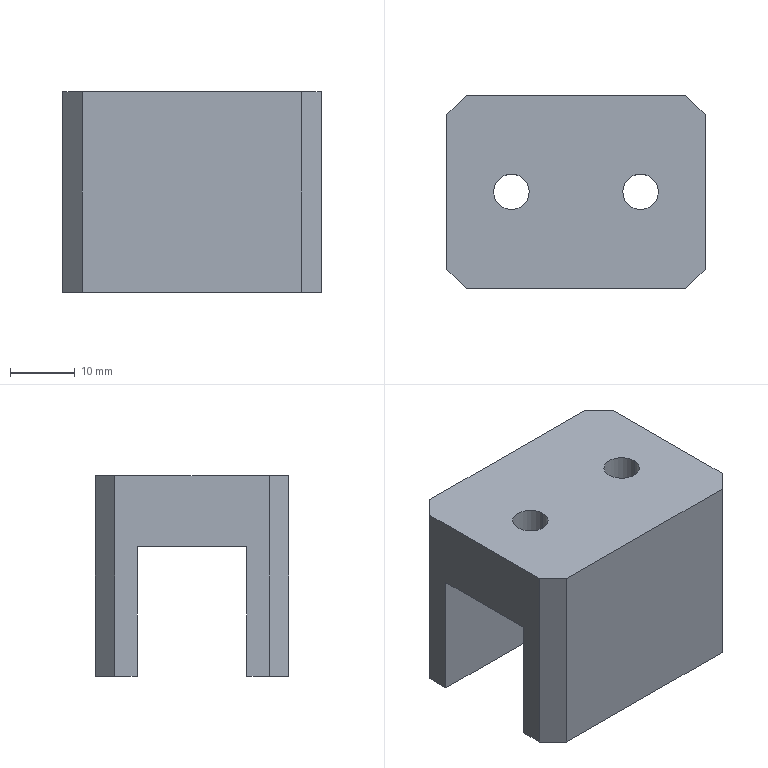Part | Creo | 1 solid | 24 faces | box 40 x 30 x 31 mm | volume 21954 mm3 | plane 16 | cylinder 8 | commonest cylinder face diameters 5.5 x4 9.5 x4
STEP:
#1=CARTESIAN_POINT('',(0.,0.,0.));
#2=DIRECTION('',(0.,0.,1.));
#3=DIRECTION('',(1.,0.,0.));
#4=AXIS2_PLACEMENT_3D('',#1,#2,#3);
#5=CARTESIAN_POINT('',(-118.,-142.,31.5));
#6=VERTEX_POINT('',#5);
#7=CARTESIAN_POINT('',(-152.,-142.,31.5));
#8=VERTEX_POINT('',#7);
#9=CARTESIAN_POINT('',(-118.,-142.,31.5));
#10=DIRECTION('',(-1.,0.,0.));
#11=VECTOR('',#10,34.);
#12=LINE('',#9,#11);
#13=EDGE_CURVE('',#6,#8,#12,.T.);
#14=ORIENTED_EDGE('',*,*,#13,.F.);
#15=CARTESIAN_POINT('',(-115.,-145.,31.5));
#16=VERTEX_POINT('',#15);
#17=CARTESIAN_POINT('',(-115.,-145.,31.5));
#18=DIRECTION('',(-0.7071,0.7071,0.));
#19=VECTOR('',#18,4.243);
#20=LINE('',#17,#19);
#21=EDGE_CURVE('',#16,#6,#20,.T.);
#22=ORIENTED_EDGE('',*,*,#21,.F.);
#23=CARTESIAN_POINT('',(-115.,-169.,31.5));
#24=VERTEX_POINT('',#23);
#25=CARTESIAN_POINT('',(-115.,-169.,31.5));
#26=DIRECTION('',(0.,1.,0.));
#27=VECTOR('',#26,24.);
#28=LINE('',#25,#27);
#29=EDGE_CURVE('',#24,#16,#28,.T.);
#30=ORIENTED_EDGE('',*,*,#29,.F.);
#31=CARTESIAN_POINT('',(-118.,-172.,31.5));
#32=VERTEX_POINT('',#31);
#33=CARTESIAN_POINT('',(-118.,-172.,31.5));
#34=DIRECTION('',(0.7071,0.7071,0.));
#35=VECTOR('',#34,4.243);
#36=LINE('',#33,#35);
#37=EDGE_CURVE('',#32,#24,#36,.T.);
#38=ORIENTED_EDGE('',*,*,#37,.F.);
#39=CARTESIAN_POINT('',(-152.,-172.,31.5));
#40=VERTEX_POINT('',#39);
#41=CARTESIAN_POINT('',(-152.,-172.,31.5));
#42=DIRECTION('',(1.,0.,0.));
#43=VECTOR('',#42,34.);
#44=LINE('',#41,#43);
#45=EDGE_CURVE('',#40,#32,#44,.T.);
#46=ORIENTED_EDGE('',*,*,#45,.F.);
#47=CARTESIAN_POINT('',(-155.,-169.,31.5));
#48=VERTEX_POINT('',#47);
#49=CARTESIAN_POINT('',(-155.,-169.,31.5));
#50=DIRECTION('',(0.7071,-0.7071,0.));
#51=VECTOR('',#50,4.243);
#52=LINE('',#49,#51);
#53=EDGE_CURVE('',#48,#40,#52,.T.);
#54=ORIENTED_EDGE('',*,*,#53,.F.);
#55=CARTESIAN_POINT('',(-155.,-145.,31.5));
#56=VERTEX_POINT('',#55);
#57=CARTESIAN_POINT('',(-155.,-145.,31.5));
#58=DIRECTION('',(0.,-1.,0.));
#59=VECTOR('',#58,24.);
#60=LINE('',#57,#59);
#61=EDGE_CURVE('',#56,#48,#60,.T.);
#62=ORIENTED_EDGE('',*,*,#61,.F.);
#63=CARTESIAN_POINT('',(-152.,-142.,31.5));
#64=DIRECTION('',(-0.7071,-0.7071,0.));
#65=VECTOR('',#64,4.243);
#66=LINE('',#63,#65);
#67=EDGE_CURVE('',#8,#56,#66,.T.);
#68=ORIENTED_EDGE('',*,*,#67,.F.);
#69=EDGE_LOOP('',(#14,#22,#30,#38,#46,#54,#62,#68));
#70=FACE_OUTER_BOUND('',#69,.F.);
#71=CARTESIAN_POINT('',(-127.75,-157.,31.5));
#72=VERTEX_POINT('',#71);
#73=CARTESIAN_POINT('',(-122.25,-157.,31.5));
#74=VERTEX_POINT('',#73);
#75=CARTESIAN_POINT('',(-125.,-157.,31.5));
#76=DIRECTION('',(0.,0.,-1.));
#77=DIRECTION('',(-1.,0.,0.));
#78=AXIS2_PLACEMENT_3D('',#75,#76,#77);
#79=CIRCLE('',#78,2.75);
#80=EDGE_CURVE('',#72,#74,#79,.T.);
#81=ORIENTED_EDGE('',*,*,#80,.F.);
#82=CARTESIAN_POINT('',(-125.,-157.,31.5));
#83=DIRECTION('',(0.,0.,-1.));
#84=DIRECTION('',(1.,0.,0.));
#85=AXIS2_PLACEMENT_3D('',#82,#83,#84);
#86=CIRCLE('',#85,2.75);
#87=EDGE_CURVE('',#74,#72,#86,.T.);
#88=ORIENTED_EDGE('',*,*,#87,.F.);
#89=EDGE_LOOP('',(#81,#88));
#90=FACE_BOUND('',#89,.F.);
#91=CARTESIAN_POINT('',(-147.75,-157.,31.5));
#92=VERTEX_POINT('',#91);
#93=CARTESIAN_POINT('',(-142.25,-157.,31.5));
#94=VERTEX_POINT('',#93);
#95=CARTESIAN_POINT('',(-145.,-157.,31.5));
#96=DIRECTION('',(0.,0.,-1.));
#97=DIRECTION('',(-1.,0.,0.));
#98=AXIS2_PLACEMENT_3D('',#95,#96,#97);
#99=CIRCLE('',#98,2.75);
#100=EDGE_CURVE('',#92,#94,#99,.T.);
#101=ORIENTED_EDGE('',*,*,#100,.F.);
#102=CARTESIAN_POINT('',(-145.,-157.,31.5));
#103=DIRECTION('',(0.,0.,-1.));
#104=DIRECTION('',(1.,0.,0.));
#105=AXIS2_PLACEMENT_3D('',#102,#103,#104);
#106=CIRCLE('',#105,2.75);
#107=EDGE_CURVE('',#94,#92,#106,.T.);
#108=ORIENTED_EDGE('',*,*,#107,.F.);
#109=EDGE_LOOP('',(#101,#108));
#110=FACE_BOUND('',#109,.F.);
#111=CARTESIAN_POINT('',(0.,-314.,31.5));
#112=DIRECTION('',(0.,0.,-1.));
#113=DIRECTION('',(-1.,0.,0.));
#114=AXIS2_PLACEMENT_3D('',#111,#112,#113);
#115=PLANE('',#114);
#116=ADVANCED_FACE('',(#70,#90,#110),#115,.F.);
#117=ORIENTED_EDGE('',*,*,#100,.T.);
#118=CARTESIAN_POINT('',(-142.25,-157.,26.5));
#119=VERTEX_POINT('',#118);
#120=CARTESIAN_POINT('',(-142.25,-157.,31.5));
#121=DIRECTION('',(0.,0.,-1.));
#122=VECTOR('',#121,5.);
#123=LINE('',#120,#122);
#124=EDGE_CURVE('',#94,#119,#123,.T.);
#125=ORIENTED_EDGE('',*,*,#124,.T.);
#126=CARTESIAN_POINT('',(-147.75,-157.,26.5));
#127=VERTEX_POINT('',#126);
#128=CARTESIAN_POINT('',(-145.,-157.,26.5));
#129=DIRECTION('',(0.,0.,1.));
#130=DIRECTION('',(1.,0.,0.));
#131=AXIS2_PLACEMENT_3D('',#128,#129,#130);
#132=CIRCLE('',#131,2.75);
#133=EDGE_CURVE('',#119,#127,#132,.T.);
#134=ORIENTED_EDGE('',*,*,#133,.T.);
#135=CARTESIAN_POINT('',(-147.75,-157.,31.5));
#136=DIRECTION('',(0.,0.,-1.));
#137=VECTOR('',#136,5.);
#138=LINE('',#135,#137);
#139=EDGE_CURVE('',#92,#127,#138,.T.);
#140=ORIENTED_EDGE('',*,*,#139,.F.);
#141=EDGE_LOOP('',(#117,#125,#134,#140));
#142=FACE_OUTER_BOUND('',#141,.F.);
#143=CARTESIAN_POINT('',(-145.,-157.,20.5));
#144=DIRECTION('',(0.,0.,-1.));
#145=DIRECTION('',(-1.,0.,0.));
#146=AXIS2_PLACEMENT_3D('',#143,#144,#145);
#147=CYLINDRICAL_SURFACE('',#146,2.75);
#148=ADVANCED_FACE('',(#142),#147,.F.);
#149=ORIENTED_EDGE('',*,*,#107,.T.);
#150=ORIENTED_EDGE('',*,*,#139,.T.);
#151=CARTESIAN_POINT('',(-145.,-157.,26.5));
#152=DIRECTION('',(0.,0.,1.));
#153=DIRECTION('',(-1.,0.,0.));
#154=AXIS2_PLACEMENT_3D('',#151,#152,#153);
#155=CIRCLE('',#154,2.75);
#156=EDGE_CURVE('',#127,#119,#155,.T.);
#157=ORIENTED_EDGE('',*,*,#156,.T.);
#158=ORIENTED_EDGE('',*,*,#124,.F.);
#159=EDGE_LOOP('',(#149,#150,#157,#158));
#160=FACE_OUTER_BOUND('',#159,.F.);
#161=CARTESIAN_POINT('',(-145.,-157.,20.5));
#162=DIRECTION('',(0.,0.,-1.));
#163=DIRECTION('',(-1.,0.,0.));
#164=AXIS2_PLACEMENT_3D('',#161,#162,#163);
#165=CYLINDRICAL_SURFACE('',#164,2.75);
#166=ADVANCED_FACE('',(#160),#165,.F.);
#167=CARTESIAN_POINT('',(-149.75,-157.,26.5));
#168=VERTEX_POINT('',#167);
#169=CARTESIAN_POINT('',(-140.25,-157.,26.5));
#170=VERTEX_POINT('',#169);
#171=CARTESIAN_POINT('',(-145.,-157.,26.5));
#172=DIRECTION('',(0.,0.,-1.));
#173=DIRECTION('',(-1.,0.,0.));
#174=AXIS2_PLACEMENT_3D('',#171,#172,#173);
#175=CIRCLE('',#174,4.75);
#176=EDGE_CURVE('',#168,#170,#175,.T.);
#177=ORIENTED_EDGE('',*,*,#176,.F.);
#178=CARTESIAN_POINT('',(-145.,-157.,26.5));
#179=DIRECTION('',(0.,0.,-1.));
#180=DIRECTION('',(1.,0.,0.));
#181=AXIS2_PLACEMENT_3D('',#178,#179,#180);
#182=CIRCLE('',#181,4.75);
#183=EDGE_CURVE('',#170,#168,#182,.T.);
#184=ORIENTED_EDGE('',*,*,#183,.F.);
#185=EDGE_LOOP('',(#177,#184));
#186=FACE_OUTER_BOUND('',#185,.F.);
#187=ORIENTED_EDGE('',*,*,#156,.F.);
#188=ORIENTED_EDGE('',*,*,#133,.F.);
#189=EDGE_LOOP('',(#187,#188));
#190=FACE_BOUND('',#189,.F.);
#191=CARTESIAN_POINT('',(-145.,-152.25,26.5));
#192=DIRECTION('',(0.,0.,1.));
#193=DIRECTION('',(1.,0.,0.));
#194=AXIS2_PLACEMENT_3D('',#191,#192,#193);
#195=PLANE('',#194);
#196=ADVANCED_FACE('',(#186,#190),#195,.F.);
#197=ORIENTED_EDGE('',*,*,#176,.T.);
#198=CARTESIAN_POINT('',(-140.25,-157.,20.5));
#199=VERTEX_POINT('',#198);
#200=CARTESIAN_POINT('',(-140.25,-157.,26.5));
#201=DIRECTION('',(0.,0.,-1.));
#202=VECTOR('',#201,6.);
#203=LINE('',#200,#202);
#204=EDGE_CURVE('',#170,#199,#203,.T.);
#205=ORIENTED_EDGE('',*,*,#204,.T.);
#206=CARTESIAN_POINT('',(-149.75,-157.,20.5));
#207=VERTEX_POINT('',#206);
#208=CARTESIAN_POINT('',(-145.,-157.,20.5));
#209=DIRECTION('',(0.,0.,1.));
#210=DIRECTION('',(1.,0.,0.));
#211=AXIS2_PLACEMENT_3D('',#208,#209,#210);
#212=CIRCLE('',#211,4.75);
#213=EDGE_CURVE('',#199,#207,#212,.T.);
#214=ORIENTED_EDGE('',*,*,#213,.T.);
#215=CARTESIAN_POINT('',(-149.75,-157.,26.5));
#216=DIRECTION('',(0.,0.,-1.));
#217=VECTOR('',#216,6.);
#218=LINE('',#215,#217);
#219=EDGE_CURVE('',#168,#207,#218,.T.);
#220=ORIENTED_EDGE('',*,*,#219,.F.);
#221=EDGE_LOOP('',(#197,#205,#214,#220));
#222=FACE_OUTER_BOUND('',#221,.F.);
#223=CARTESIAN_POINT('',(-145.,-157.,20.5));
#224=DIRECTION('',(0.,0.,-1.));
#225=DIRECTION('',(-1.,0.,0.));
#226=AXIS2_PLACEMENT_3D('',#223,#224,#225);
#227=CYLINDRICAL_SURFACE('',#226,4.75);
#228=ADVANCED_FACE('',(#222),#227,.F.);
#229=ORIENTED_EDGE('',*,*,#183,.T.);
#230=ORIENTED_EDGE('',*,*,#219,.T.);
#231=CARTESIAN_POINT('',(-145.,-157.,20.5));
#232=DIRECTION('',(0.,0.,1.));
#233=DIRECTION('',(-1.,0.,0.));
#234=AXIS2_PLACEMENT_3D('',#231,#232,#233);
#235=CIRCLE('',#234,4.75);
#236=EDGE_CURVE('',#207,#199,#235,.T.);
#237=ORIENTED_EDGE('',*,*,#236,.T.);
#238=ORIENTED_EDGE('',*,*,#204,.F.);
#239=EDGE_LOOP('',(#229,#230,#237,#238));
#240=FACE_OUTER_BOUND('',#239,.F.);
#241=CARTESIAN_POINT('',(-145.,-157.,20.5));
#242=DIRECTION('',(0.,0.,-1.));
#243=DIRECTION('',(-1.,0.,0.));
#244=AXIS2_PLACEMENT_3D('',#241,#242,#243);
#245=CYLINDRICAL_SURFACE('',#244,4.75);
#246=ADVANCED_FACE('',(#240),#245,.F.);
#247=CARTESIAN_POINT('',(-155.,-148.5,20.5));
#248=VERTEX_POINT('',#247);
#249=CARTESIAN_POINT('',(-155.,-165.5,20.5));
#250=VERTEX_POINT('',#249);
#251=CARTESIAN_POINT('',(-155.,-148.5,20.5));
#252=DIRECTION('',(0.,-1.,0.));
#253=VECTOR('',#252,17.);
#254=LINE('',#251,#253);
#255=EDGE_CURVE('',#248,#250,#254,.T.);
#256=ORIENTED_EDGE('',*,*,#255,.T.);
#257=CARTESIAN_POINT('',(-115.,-165.5,20.5));
#258=VERTEX_POINT('',#257);
#259=CARTESIAN_POINT('',(-115.,-165.5,20.5));
#260=DIRECTION('',(-1.,0.,0.));
#261=VECTOR('',#260,40.);
#262=LINE('',#259,#261);
#263=EDGE_CURVE('',#258,#250,#262,.T.);
#264=ORIENTED_EDGE('',*,*,#263,.F.);
#265=CARTESIAN_POINT('',(-115.,-148.5,20.5));
#266=VERTEX_POINT('',#265);
#267=CARTESIAN_POINT('',(-115.,-165.5,20.5));
#268=DIRECTION('',(0.,1.,0.));
#269=VECTOR('',#268,17.);
#270=LINE('',#267,#269);
#271=EDGE_CURVE('',#258,#266,#270,.T.);
#272=ORIENTED_EDGE('',*,*,#271,.T.);
#273=CARTESIAN_POINT('',(-155.,-148.5,20.5));
#274=DIRECTION('',(1.,0.,0.));
#275=VECTOR('',#274,40.);
#276=LINE('',#273,#275);
#277=EDGE_CURVE('',#248,#266,#276,.T.);
#278=ORIENTED_EDGE('',*,*,#277,.F.);
#279=EDGE_LOOP('',(#256,#264,#272,#278));
#280=FACE_OUTER_BOUND('',#279,.F.);
#281=CARTESIAN_POINT('',(-129.75,-157.,20.5));
#282=VERTEX_POINT('',#281);
#283=CARTESIAN_POINT('',(-120.25,-157.,20.5));
#284=VERTEX_POINT('',#283);
#285=CARTESIAN_POINT('',(-125.,-157.,20.5));
#286=DIRECTION('',(0.,0.,1.));
#287=DIRECTION('',(-1.,0.,0.));
#288=AXIS2_PLACEMENT_3D('',#285,#286,#287);
#289=CIRCLE('',#288,4.75);
#290=EDGE_CURVE('',#282,#284,#289,.T.);
#291=ORIENTED_EDGE('',*,*,#290,.F.);
#292=CARTESIAN_POINT('',(-125.,-157.,20.5));
#293=DIRECTION('',(0.,0.,1.));
#294=DIRECTION('',(1.,0.,0.));
#295=AXIS2_PLACEMENT_3D('',#292,#293,#294);
#296=CIRCLE('',#295,4.75);
#297=EDGE_CURVE('',#284,#282,#296,.T.);
#298=ORIENTED_EDGE('',*,*,#297,.F.);
#299=EDGE_LOOP('',(#291,#298));
#300=FACE_BOUND('',#299,.F.);
#301=ORIENTED_EDGE('',*,*,#236,.F.);
#302=ORIENTED_EDGE('',*,*,#213,.F.);
#303=EDGE_LOOP('',(#301,#302));
#304=FACE_BOUND('',#303,.F.);
#305=CARTESIAN_POINT('',(0.,-314.,20.5));
#306=DIRECTION('',(0.,0.,1.));
#307=DIRECTION('',(1.,0.,0.));
#308=AXIS2_PLACEMENT_3D('',#305,#306,#307);
#309=PLANE('',#308);
#310=ADVANCED_FACE('',(#280,#300,#304),#309,.F.);
#311=CARTESIAN_POINT('',(-120.25,-157.,26.5));
#312=VERTEX_POINT('',#311);
#313=CARTESIAN_POINT('',(-129.75,-157.,26.5));
#314=VERTEX_POINT('',#313);
#315=CARTESIAN_POINT('',(-125.,-157.,26.5));
#316=DIRECTION('',(0.,0.,-1.));
#317=DIRECTION('',(1.,0.,0.));
#318=AXIS2_PLACEMENT_3D('',#315,#316,#317);
#319=CIRCLE('',#318,4.75);
#320=EDGE_CURVE('',#312,#314,#319,.T.);
#321=ORIENTED_EDGE('',*,*,#320,.T.);
#322=CARTESIAN_POINT('',(-129.75,-157.,26.5));
#323=DIRECTION('',(0.,0.,-1.));
#324=VECTOR('',#323,6.);
#325=LINE('',#322,#324);
#326=EDGE_CURVE('',#314,#282,#325,.T.);
#327=ORIENTED_EDGE('',*,*,#326,.T.);
#328=ORIENTED_EDGE('',*,*,#290,.T.);
#329=CARTESIAN_POINT('',(-120.25,-157.,26.5));
#330=DIRECTION('',(0.,0.,-1.));
#331=VECTOR('',#330,6.);
#332=LINE('',#329,#331);
#333=EDGE_CURVE('',#312,#284,#332,.T.);
#334=ORIENTED_EDGE('',*,*,#333,.F.);
#335=EDGE_LOOP('',(#321,#327,#328,#334));
#336=FACE_OUTER_BOUND('',#335,.F.);
#337=CARTESIAN_POINT('',(-125.,-157.,20.5));
#338=DIRECTION('',(0.,0.,-1.));
#339=DIRECTION('',(-1.,0.,0.));
#340=AXIS2_PLACEMENT_3D('',#337,#338,#339);
#341=CYLINDRICAL_SURFACE('',#340,4.75);
#342=ADVANCED_FACE('',(#336),#341,.F.);
#343=CARTESIAN_POINT('',(-125.,-157.,26.5));
#344=DIRECTION('',(0.,0.,-1.));
#345=DIRECTION('',(-1.,0.,0.));
#346=AXIS2_PLACEMENT_3D('',#343,#344,#345);
#347=CIRCLE('',#346,4.75);
#348=EDGE_CURVE('',#314,#312,#347,.T.);
#349=ORIENTED_EDGE('',*,*,#348,.F.);
#350=ORIENTED_EDGE('',*,*,#320,.F.);
#351=EDGE_LOOP('',(#349,#350));
#352=FACE_OUTER_BOUND('',#351,.F.);
#353=CARTESIAN_POINT('',(-127.75,-157.,26.5));
#354=VERTEX_POINT('',#353);
#355=CARTESIAN_POINT('',(-122.25,-157.,26.5));
#356=VERTEX_POINT('',#355);
#357=CARTESIAN_POINT('',(-125.,-157.,26.5));
#358=DIRECTION('',(0.,0.,1.));
#359=DIRECTION('',(-1.,0.,0.));
#360=AXIS2_PLACEMENT_3D('',#357,#358,#359);
#361=CIRCLE('',#360,2.75);
#362=EDGE_CURVE('',#354,#356,#361,.T.);
#363=ORIENTED_EDGE('',*,*,#362,.F.);
#364=CARTESIAN_POINT('',(-125.,-157.,26.5));
#365=DIRECTION('',(0.,0.,1.));
#366=DIRECTION('',(1.,0.,0.));
#367=AXIS2_PLACEMENT_3D('',#364,#365,#366);
#368=CIRCLE('',#367,2.75);
#369=EDGE_CURVE('',#356,#354,#368,.T.);
#370=ORIENTED_EDGE('',*,*,#369,.F.);
#371=EDGE_LOOP('',(#363,#370));
#372=FACE_BOUND('',#371,.F.);
#373=CARTESIAN_POINT('',(-125.,-152.25,26.5));
#374=DIRECTION('',(0.,0.,1.));
#375=DIRECTION('',(1.,0.,0.));
#376=AXIS2_PLACEMENT_3D('',#373,#374,#375);
#377=PLANE('',#376);
#378=ADVANCED_FACE('',(#352,#372),#377,.F.);
#379=ORIENTED_EDGE('',*,*,#87,.T.);
#380=CARTESIAN_POINT('',(-127.75,-157.,31.5));
#381=DIRECTION('',(0.,0.,-1.));
#382=VECTOR('',#381,5.);
#383=LINE('',#380,#382);
#384=EDGE_CURVE('',#72,#354,#383,.T.);
#385=ORIENTED_EDGE('',*,*,#384,.T.);
#386=ORIENTED_EDGE('',*,*,#362,.T.);
#387=CARTESIAN_POINT('',(-122.25,-157.,31.5));
#388=DIRECTION('',(0.,0.,-1.));
#389=VECTOR('',#388,5.);
#390=LINE('',#387,#389);
#391=EDGE_CURVE('',#74,#356,#390,.T.);
#392=ORIENTED_EDGE('',*,*,#391,.F.);
#393=EDGE_LOOP('',(#379,#385,#386,#392));
#394=FACE_OUTER_BOUND('',#393,.F.);
#395=CARTESIAN_POINT('',(-125.,-157.,20.5));
#396=DIRECTION('',(0.,0.,-1.));
#397=DIRECTION('',(-1.,0.,0.));
#398=AXIS2_PLACEMENT_3D('',#395,#396,#397);
#399=CYLINDRICAL_SURFACE('',#398,2.75);
#400=ADVANCED_FACE('',(#394),#399,.F.);
#401=ORIENTED_EDGE('',*,*,#80,.T.);
#402=ORIENTED_EDGE('',*,*,#391,.T.);
#403=ORIENTED_EDGE('',*,*,#369,.T.);
#404=ORIENTED_EDGE('',*,*,#384,.F.);
#405=EDGE_LOOP('',(#401,#402,#403,#404));
#406=FACE_OUTER_BOUND('',#405,.F.);
#407=CARTESIAN_POINT('',(-125.,-157.,20.5));
#408=DIRECTION('',(0.,0.,-1.));
#409=DIRECTION('',(-1.,0.,0.));
#410=AXIS2_PLACEMENT_3D('',#407,#408,#409);
#411=CYLINDRICAL_SURFACE('',#410,2.75);
#412=ADVANCED_FACE('',(#406),#411,.F.);
#413=ORIENTED_EDGE('',*,*,#348,.T.);
#414=ORIENTED_EDGE('',*,*,#333,.T.);
#415=ORIENTED_EDGE('',*,*,#297,.T.);
#416=ORIENTED_EDGE('',*,*,#326,.F.);
#417=EDGE_LOOP('',(#413,#414,#415,#416));
#418=FACE_OUTER_BOUND('',#417,.F.);
#419=CARTESIAN_POINT('',(-125.,-157.,20.5));
#420=DIRECTION('',(0.,0.,-1.));
#421=DIRECTION('',(-1.,0.,0.));
#422=AXIS2_PLACEMENT_3D('',#419,#420,#421);
#423=CYLINDRICAL_SURFACE('',#422,4.75);
#424=ADVANCED_FACE('',(#418),#423,.F.);
#425=ORIENTED_EDGE('',*,*,#61,.T.);
#426=CARTESIAN_POINT('',(-155.,-169.,0.5));
#427=VERTEX_POINT('',#426);
#428=CARTESIAN_POINT('',(-155.,-169.,31.5));
#429=DIRECTION('',(0.,0.,-1.));
#430=VECTOR('',#429,31.);
#431=LINE('',#428,#430);
#432=EDGE_CURVE('',#48,#427,#431,.T.);
#433=ORIENTED_EDGE('',*,*,#432,.T.);
#434=CARTESIAN_POINT('',(-155.,-165.5,0.5));
#435=VERTEX_POINT('',#434);
#436=CARTESIAN_POINT('',(-155.,-165.5,0.5));
#437=DIRECTION('',(0.,-1.,0.));
#438=VECTOR('',#437,3.5);
#439=LINE('',#436,#438);
#440=EDGE_CURVE('',#435,#427,#439,.T.);
#441=ORIENTED_EDGE('',*,*,#440,.F.);
#442=CARTESIAN_POINT('',(-155.,-165.5,20.5));
#443=DIRECTION('',(0.,0.,-1.));
#444=VECTOR('',#443,20.);
#445=LINE('',#442,#444);
#446=EDGE_CURVE('',#250,#435,#445,.T.);
#447=ORIENTED_EDGE('',*,*,#446,.F.);
#448=ORIENTED_EDGE('',*,*,#255,.F.);
#449=CARTESIAN_POINT('',(-155.,-148.5,0.5));
#450=VERTEX_POINT('',#449);
#451=CARTESIAN_POINT('',(-155.,-148.5,20.5));
#452=DIRECTION('',(0.,0.,-1.));
#453=VECTOR('',#452,20.);
#454=LINE('',#451,#453);
#455=EDGE_CURVE('',#248,#450,#454,.T.);
#456=ORIENTED_EDGE('',*,*,#455,.T.);
#457=CARTESIAN_POINT('',(-155.,-145.,0.5));
#458=VERTEX_POINT('',#457);
#459=CARTESIAN_POINT('',(-155.,-145.,0.5));
#460=DIRECTION('',(0.,-1.,0.));
#461=VECTOR('',#460,3.5);
#462=LINE('',#459,#461);
#463=EDGE_CURVE('',#458,#450,#462,.T.);
#464=ORIENTED_EDGE('',*,*,#463,.F.);
#465=CARTESIAN_POINT('',(-155.,-145.,0.5));
#466=DIRECTION('',(0.,0.,1.));
#467=VECTOR('',#466,31.);
#468=LINE('',#465,#467);
#469=EDGE_CURVE('',#458,#56,#468,.T.);
#470=ORIENTED_EDGE('',*,*,#469,.T.);
#471=EDGE_LOOP('',(#425,#433,#441,#447,#448,#456,#464,#470));
#472=FACE_OUTER_BOUND('',#471,.F.);
#473=CARTESIAN_POINT('',(-155.,-172.,0.5));
#474=DIRECTION('',(1.,0.,0.));
#475=DIRECTION('',(0.,0.,-1.));
#476=AXIS2_PLACEMENT_3D('',#473,#474,#475);
#477=PLANE('',#476);
#478=ADVANCED_FACE('',(#472),#477,.F.);
#479=CARTESIAN_POINT('',(-152.,-172.,0.5));
#480=VERTEX_POINT('',#479);
#481=CARTESIAN_POINT('',(-152.,-172.,0.5));
#482=DIRECTION('',(-0.7071,0.7071,0.));
#483=VECTOR('',#482,4.243);
#484=LINE('',#481,#483);
#485=EDGE_CURVE('',#480,#427,#484,.T.);
#486=ORIENTED_EDGE('',*,*,#485,.T.);
#487=ORIENTED_EDGE('',*,*,#432,.F.);
#488=ORIENTED_EDGE('',*,*,#53,.T.);
#489=CARTESIAN_POINT('',(-152.,-172.,0.5));
#490=DIRECTION('',(0.,0.,1.));
#491=VECTOR('',#490,31.);
#492=LINE('',#489,#491);
#493=EDGE_CURVE('',#480,#40,#492,.T.);
#494=ORIENTED_EDGE('',*,*,#493,.F.);
#495=EDGE_LOOP('',(#486,#487,#488,#494));
#496=FACE_OUTER_BOUND('',#495,.F.);
#497=CARTESIAN_POINT('',(-155.,-169.,0.5));
#498=DIRECTION('',(0.7071,0.7071,0.));
#499=DIRECTION('',(0.,0.,1.));
#500=AXIS2_PLACEMENT_3D('',#497,#498,#499);
#501=PLANE('',#500);
#502=ADVANCED_FACE('',(#496),#501,.F.);
#503=CARTESIAN_POINT('',(-115.,-169.,0.5));
#504=VERTEX_POINT('',#503);
#505=CARTESIAN_POINT('',(-115.,-165.5,0.5));
#506=VERTEX_POINT('',#505);
#507=CARTESIAN_POINT('',(-115.,-169.,0.5));
#508=DIRECTION('',(0.,1.,0.));
#509=VECTOR('',#508,3.5);
#510=LINE('',#507,#509);
#511=EDGE_CURVE('',#504,#506,#510,.T.);
#512=ORIENTED_EDGE('',*,*,#511,.T.);
#513=CARTESIAN_POINT('',(-155.,-165.5,0.5));
#514=DIRECTION('',(1.,0.,0.));
#515=VECTOR('',#514,40.);
#516=LINE('',#513,#515);
#517=EDGE_CURVE('',#435,#506,#516,.T.);
#518=ORIENTED_EDGE('',*,*,#517,.F.);
#519=ORIENTED_EDGE('',*,*,#440,.T.);
#520=ORIENTED_EDGE('',*,*,#485,.F.);
#521=CARTESIAN_POINT('',(-118.,-172.,0.5));
#522=VERTEX_POINT('',#521);
#523=CARTESIAN_POINT('',(-152.,-172.,0.5));
#524=DIRECTION('',(1.,0.,0.));
#525=VECTOR('',#524,34.);
#526=LINE('',#523,#525);
#527=EDGE_CURVE('',#480,#522,#526,.T.);
#528=ORIENTED_EDGE('',*,*,#527,.T.);
#529=CARTESIAN_POINT('',(-115.,-169.,0.5));
#530=DIRECTION('',(-0.7071,-0.7071,0.));
#531=VECTOR('',#530,4.243);
#532=LINE('',#529,#531);
#533=EDGE_CURVE('',#504,#522,#532,.T.);
#534=ORIENTED_EDGE('',*,*,#533,.F.);
#535=EDGE_LOOP('',(#512,#518,#519,#520,#528,#534));
#536=FACE_OUTER_BOUND('',#535,.F.);
#537=CARTESIAN_POINT('',(0.,-314.,0.5));
#538=DIRECTION('',(0.,0.,-1.));
#539=DIRECTION('',(-1.,0.,0.));
#540=AXIS2_PLACEMENT_3D('',#537,#538,#539);
#541=PLANE('',#540);
#542=ADVANCED_FACE('',(#536),#541,.T.);
#543=CARTESIAN_POINT('',(-115.,-148.5,0.5));
#544=VERTEX_POINT('',#543);
#545=CARTESIAN_POINT('',(-115.,-145.,0.5));
#546=VERTEX_POINT('',#545);
#547=CARTESIAN_POINT('',(-115.,-148.5,0.5));
#548=DIRECTION('',(0.,1.,0.));
#549=VECTOR('',#548,3.5);
#550=LINE('',#547,#549);
#551=EDGE_CURVE('',#544,#546,#550,.T.);
#552=ORIENTED_EDGE('',*,*,#551,.F.);
#553=CARTESIAN_POINT('',(-115.,-148.5,20.5));
#554=DIRECTION('',(0.,0.,-1.));
#555=VECTOR('',#554,20.);
#556=LINE('',#553,#555);
#557=EDGE_CURVE('',#266,#544,#556,.T.);
#558=ORIENTED_EDGE('',*,*,#557,.F.);
#559=ORIENTED_EDGE('',*,*,#271,.F.);
#560=CARTESIAN_POINT('',(-115.,-165.5,20.5));
#561=DIRECTION('',(0.,0.,-1.));
#562=VECTOR('',#561,20.);
#563=LINE('',#560,#562);
#564=EDGE_CURVE('',#258,#506,#563,.T.);
#565=ORIENTED_EDGE('',*,*,#564,.T.);
#566=ORIENTED_EDGE('',*,*,#511,.F.);
#567=CARTESIAN_POINT('',(-115.,-169.,0.5));
#568=DIRECTION('',(0.,0.,1.));
#569=VECTOR('',#568,31.);
#570=LINE('',#567,#569);
#571=EDGE_CURVE('',#504,#24,#570,.T.);
#572=ORIENTED_EDGE('',*,*,#571,.T.);
#573=ORIENTED_EDGE('',*,*,#29,.T.);
#574=CARTESIAN_POINT('',(-115.,-145.,31.5));
#575=DIRECTION('',(0.,0.,-1.));
#576=VECTOR('',#575,31.);
#577=LINE('',#574,#576);
#578=EDGE_CURVE('',#16,#546,#577,.T.);
#579=ORIENTED_EDGE('',*,*,#578,.T.);
#580=EDGE_LOOP('',(#552,#558,#559,#565,#566,#572,#573,#579));
#581=FACE_OUTER_BOUND('',#580,.F.);
#582=CARTESIAN_POINT('',(-115.,-142.,0.5));
#583=DIRECTION('',(-1.,0.,0.));
#584=DIRECTION('',(0.,-1.,0.));
#585=AXIS2_PLACEMENT_3D('',#582,#583,#584);
#586=PLANE('',#585);
#587=ADVANCED_FACE('',(#581),#586,.F.);
#588=ORIENTED_EDGE('',*,*,#463,.T.);
#589=CARTESIAN_POINT('',(-115.,-148.5,0.5));
#590=DIRECTION('',(-1.,0.,0.));
#591=VECTOR('',#590,40.);
#592=LINE('',#589,#591);
#593=EDGE_CURVE('',#544,#450,#592,.T.);
#594=ORIENTED_EDGE('',*,*,#593,.F.);
#595=ORIENTED_EDGE('',*,*,#551,.T.);
#596=CARTESIAN_POINT('',(-118.,-142.,0.5));
#597=VERTEX_POINT('',#596);
#598=CARTESIAN_POINT('',(-118.,-142.,0.5));
#599=DIRECTION('',(0.7071,-0.7071,0.));
#600=VECTOR('',#599,4.243);
#601=LINE('',#598,#600);
#602=EDGE_CURVE('',#597,#546,#601,.T.);
#603=ORIENTED_EDGE('',*,*,#602,.F.);
#604=CARTESIAN_POINT('',(-152.,-142.,0.5));
#605=VERTEX_POINT('',#604);
#606=CARTESIAN_POINT('',(-118.,-142.,0.5));
#607=DIRECTION('',(-1.,0.,0.));
#608=VECTOR('',#607,34.);
#609=LINE('',#606,#608);
#610=EDGE_CURVE('',#597,#605,#609,.T.);
#611=ORIENTED_EDGE('',*,*,#610,.T.);
#612=CARTESIAN_POINT('',(-155.,-145.,0.5));
#613=DIRECTION('',(0.7071,0.7071,0.));
#614=VECTOR('',#613,4.243);
#615=LINE('',#612,#614);
#616=EDGE_CURVE('',#458,#605,#615,.T.);
#617=ORIENTED_EDGE('',*,*,#616,.F.);
#618=EDGE_LOOP('',(#588,#594,#595,#603,#611,#617));
#619=FACE_OUTER_BOUND('',#618,.F.);
#620=CARTESIAN_POINT('',(0.,-314.,0.5));
#621=DIRECTION('',(0.,0.,-1.));
#622=DIRECTION('',(-1.,0.,0.));
#623=AXIS2_PLACEMENT_3D('',#620,#621,#622);
#624=PLANE('',#623);
#625=ADVANCED_FACE('',(#619),#624,.T.);
#626=ORIENTED_EDGE('',*,*,#593,.T.);
#627=ORIENTED_EDGE('',*,*,#455,.F.);
#628=ORIENTED_EDGE('',*,*,#277,.T.);
#629=ORIENTED_EDGE('',*,*,#557,.T.);
#630=EDGE_LOOP('',(#626,#627,#628,#629));
#631=FACE_OUTER_BOUND('',#630,.F.);
#632=CARTESIAN_POINT('',(-115.,-148.5,-12.5));
#633=DIRECTION('',(0.,1.,0.));
#634=DIRECTION('',(0.,0.,1.));
#635=AXIS2_PLACEMENT_3D('',#632,#633,#634);
#636=PLANE('',#635);
#637=ADVANCED_FACE('',(#631),#636,.F.);
#638=ORIENTED_EDGE('',*,*,#602,.T.);
#639=ORIENTED_EDGE('',*,*,#578,.F.);
#640=ORIENTED_EDGE('',*,*,#21,.T.);
#641=CARTESIAN_POINT('',(-118.,-142.,0.5));
#642=DIRECTION('',(0.,0.,1.));
#643=VECTOR('',#642,31.);
#644=LINE('',#641,#643);
#645=EDGE_CURVE('',#597,#6,#644,.T.);
#646=ORIENTED_EDGE('',*,*,#645,.F.);
#647=EDGE_LOOP('',(#638,#639,#640,#646));
#648=FACE_OUTER_BOUND('',#647,.F.);
#649=CARTESIAN_POINT('',(-115.,-145.,0.5));
#650=DIRECTION('',(-0.7071,-0.7071,0.));
#651=DIRECTION('',(0.,0.,1.));
#652=AXIS2_PLACEMENT_3D('',#649,#650,#651);
#653=PLANE('',#652);
#654=ADVANCED_FACE('',(#648),#653,.F.);
#655=ORIENTED_EDGE('',*,*,#610,.F.);
#656=ORIENTED_EDGE('',*,*,#645,.T.);
#657=ORIENTED_EDGE('',*,*,#13,.T.);
#658=CARTESIAN_POINT('',(-152.,-142.,31.5));
#659=DIRECTION('',(0.,0.,-1.));
#660=VECTOR('',#659,31.);
#661=LINE('',#658,#660);
#662=EDGE_CURVE('',#8,#605,#661,.T.);
#663=ORIENTED_EDGE('',*,*,#662,.T.);
#664=EDGE_LOOP('',(#655,#656,#657,#663));
#665=FACE_OUTER_BOUND('',#664,.F.);
#666=CARTESIAN_POINT('',(-155.,-142.,0.5));
#667=DIRECTION('',(0.,-1.,0.));
#668=DIRECTION('',(0.,0.,-1.));
#669=AXIS2_PLACEMENT_3D('',#666,#667,#668);
#670=PLANE('',#669);
#671=ADVANCED_FACE('',(#665),#670,.F.);
#672=ORIENTED_EDGE('',*,*,#616,.T.);
#673=ORIENTED_EDGE('',*,*,#662,.F.);
#674=ORIENTED_EDGE('',*,*,#67,.T.);
#675=ORIENTED_EDGE('',*,*,#469,.F.);
#676=EDGE_LOOP('',(#672,#673,#674,#675));
#677=FACE_OUTER_BOUND('',#676,.F.);
#678=CARTESIAN_POINT('',(-152.,-142.,0.5));
#679=DIRECTION('',(0.7071,-0.7071,0.));
#680=DIRECTION('',(0.,0.,1.));
#681=AXIS2_PLACEMENT_3D('',#678,#679,#680);
#682=PLANE('',#681);
#683=ADVANCED_FACE('',(#677),#682,.F.);
#684=ORIENTED_EDGE('',*,*,#517,.T.);
#685=ORIENTED_EDGE('',*,*,#564,.F.);
#686=ORIENTED_EDGE('',*,*,#263,.T.);
#687=ORIENTED_EDGE('',*,*,#446,.T.);
#688=EDGE_LOOP('',(#684,#685,#686,#687));
#689=FACE_OUTER_BOUND('',#688,.F.);
#690=CARTESIAN_POINT('',(-155.,-165.5,-12.5));
#691=DIRECTION('',(0.,-1.,0.));
#692=DIRECTION('',(1.,0.,0.));
#693=AXIS2_PLACEMENT_3D('',#690,#691,#692);
#694=PLANE('',#693);
#695=ADVANCED_FACE('',(#689),#694,.F.);
#696=ORIENTED_EDGE('',*,*,#533,.T.);
#697=CARTESIAN_POINT('',(-118.,-172.,31.5));
#698=DIRECTION('',(0.,0.,-1.));
#699=VECTOR('',#698,31.);
#700=LINE('',#697,#699);
#701=EDGE_CURVE('',#32,#522,#700,.T.);
#702=ORIENTED_EDGE('',*,*,#701,.F.);
#703=ORIENTED_EDGE('',*,*,#37,.T.);
#704=ORIENTED_EDGE('',*,*,#571,.F.);
#705=EDGE_LOOP('',(#696,#702,#703,#704));
#706=FACE_OUTER_BOUND('',#705,.F.);
#707=CARTESIAN_POINT('',(-118.,-172.,0.5));
#708=DIRECTION('',(-0.7071,0.7071,0.));
#709=DIRECTION('',(0.,0.,1.));
#710=AXIS2_PLACEMENT_3D('',#707,#708,#709);
#711=PLANE('',#710);
#712=ADVANCED_FACE('',(#706),#711,.F.);
#713=ORIENTED_EDGE('',*,*,#527,.F.);
#714=ORIENTED_EDGE('',*,*,#493,.T.);
#715=ORIENTED_EDGE('',*,*,#45,.T.);
#716=ORIENTED_EDGE('',*,*,#701,.T.);
#717=EDGE_LOOP('',(#713,#714,#715,#716));
#718=FACE_OUTER_BOUND('',#717,.F.);
#719=CARTESIAN_POINT('',(-115.,-172.,0.5));
#720=DIRECTION('',(0.,1.,0.));
#721=DIRECTION('',(-1.,0.,0.));
#722=AXIS2_PLACEMENT_3D('',#719,#720,#721);
#723=PLANE('',#722);
#724=ADVANCED_FACE('',(#718),#723,.F.);
#725=CLOSED_SHELL('',(#116,#148,#166,#196,#228,#246,#310,#342,#378,#400,#412,#424,#478,#502,#542,#587,#625,#637,#654,#671,#683,#695,#712,#724));
#726=MANIFOLD_SOLID_BREP('',#725);
#727=(LENGTH_UNIT()NAMED_UNIT(*)SI_UNIT(.MILLI.,.METRE.));
#728=UNCERTAINTY_MEASURE_WITH_UNIT(LENGTH_MEASURE(0.005883),#727,'','');
#729=(NAMED_UNIT(*)PLANE_ANGLE_UNIT()SI_UNIT($,.RADIAN.));
#730=PLANE_ANGLE_MEASURE_WITH_UNIT(PLANE_ANGLE_MEASURE(0.01745),#729);
#731=(CONVERSION_BASED_UNIT('DEGREE',#730)NAMED_UNIT(*)PLANE_ANGLE_UNIT());
#732=(NAMED_UNIT(*)SI_UNIT($,.STERADIAN.)SOLID_ANGLE_UNIT());
#733=(GEOMETRIC_REPRESENTATION_CONTEXT(3)GLOBAL_UNCERTAINTY_ASSIGNED_CONTEXT((#728))GLOBAL_UNIT_ASSIGNED_CONTEXT((#727,#731,#732))REPRESENTATION_CONTEXT('',''));
#734=ADVANCED_BREP_SHAPE_REPRESENTATION('',(#4,#726),#733);